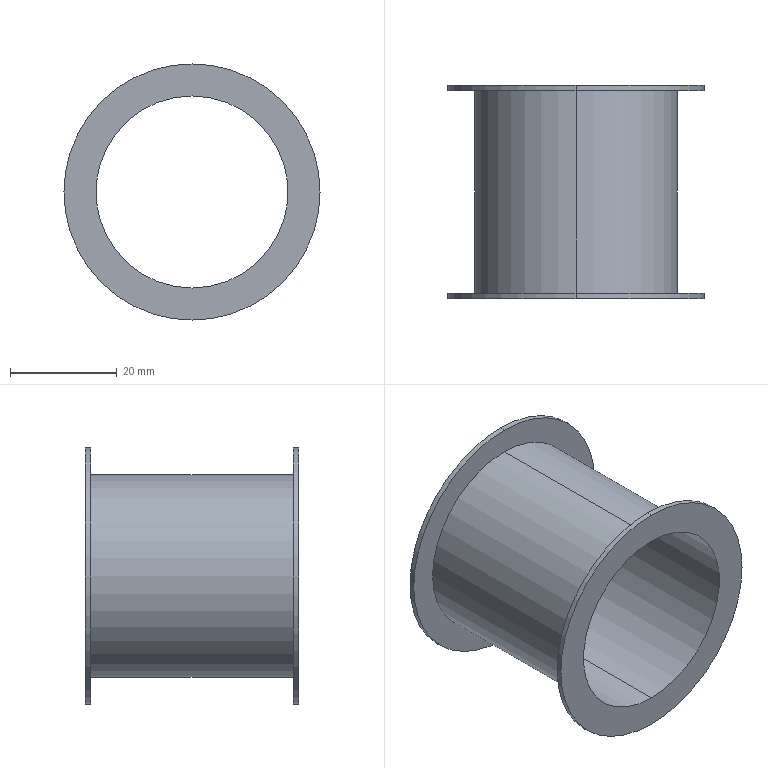Part | SolidWorks | features Revolution 1 | 1 solid | 12 faces | box 48 x 40 x 48 mm | volume 6000 mm3 | cylinder 8 | plane 4 | commonest cylinder face diameters 48 x4 36 x2 38 x2
STEP:
#1=CARTESIAN_POINT('',(0.,40.,-24.));
#2=VERTEX_POINT('',#1);
#3=CARTESIAN_POINT('',(0.,40.,24.));
#4=VERTEX_POINT('',#3);
#5=CARTESIAN_POINT('',(0.,40.,0.));
#6=DIRECTION('',(0.,-1.,0.));
#7=DIRECTION('',(0.,0.,-1.));
#8=AXIS2_PLACEMENT_3D('',#5,#6,#7);
#9=CIRCLE('',#8,24.);
#10=EDGE_CURVE('',#2,#4,#9,.T.);
#11=ORIENTED_EDGE('',*,*,#10,.T.);
#12=CARTESIAN_POINT('',(0.,39.,24.));
#13=VERTEX_POINT('',#12);
#14=CARTESIAN_POINT('',(0.,0.,24.));
#15=DIRECTION('',(0.,-1.,0.));
#16=VECTOR('',#15,1000.);
#17=LINE('',#14,#16);
#18=EDGE_CURVE('',#4,#13,#17,.T.);
#19=ORIENTED_EDGE('',*,*,#18,.T.);
#20=CARTESIAN_POINT('',(0.,39.,-24.));
#21=VERTEX_POINT('',#20);
#22=CARTESIAN_POINT('',(0.,39.,0.));
#23=DIRECTION('',(0.,-1.,0.));
#24=DIRECTION('',(0.,0.,-1.));
#25=AXIS2_PLACEMENT_3D('',#22,#23,#24);
#26=CIRCLE('',#25,24.);
#27=EDGE_CURVE('',#21,#13,#26,.T.);
#28=ORIENTED_EDGE('',*,*,#27,.F.);
#29=CARTESIAN_POINT('',(0.,0.,-24.));
#30=DIRECTION('',(0.,-1.,0.));
#31=VECTOR('',#30,1000.);
#32=LINE('',#29,#31);
#33=EDGE_CURVE('',#2,#21,#32,.T.);
#34=ORIENTED_EDGE('',*,*,#33,.F.);
#35=EDGE_LOOP('',(#11,#19,#28,#34));
#36=FACE_OUTER_BOUND('',#35,.T.);
#37=CARTESIAN_POINT('',(0.,0.,0.));
#38=DIRECTION('',(0.,-1.,0.));
#39=DIRECTION('',(0.,0.,-1.));
#40=AXIS2_PLACEMENT_3D('',#37,#38,#39);
#41=CYLINDRICAL_SURFACE('',#40,24.);
#42=ADVANCED_FACE('',(#36),#41,.T.);
#43=CARTESIAN_POINT('',(0.,39.,-19.));
#44=VERTEX_POINT('',#43);
#45=CARTESIAN_POINT('',(0.,39.,19.));
#46=VERTEX_POINT('',#45);
#47=CARTESIAN_POINT('',(0.,39.,0.));
#48=DIRECTION('',(0.,-1.,0.));
#49=DIRECTION('',(0.,0.,-1.));
#50=AXIS2_PLACEMENT_3D('',#47,#48,#49);
#51=CIRCLE('',#50,19.);
#52=EDGE_CURVE('',#44,#46,#51,.T.);
#53=ORIENTED_EDGE('',*,*,#52,.T.);
#54=CARTESIAN_POINT('',(0.,1.,19.));
#55=VERTEX_POINT('',#54);
#56=CARTESIAN_POINT('',(0.,0.,19.));
#57=DIRECTION('',(0.,-1.,0.));
#58=VECTOR('',#57,1000.);
#59=LINE('',#56,#58);
#60=EDGE_CURVE('',#46,#55,#59,.T.);
#61=ORIENTED_EDGE('',*,*,#60,.T.);
#62=CARTESIAN_POINT('',(0.,1.,-19.));
#63=VERTEX_POINT('',#62);
#64=CARTESIAN_POINT('',(0.,1.,0.));
#65=DIRECTION('',(0.,-1.,0.));
#66=DIRECTION('',(0.,0.,-1.));
#67=AXIS2_PLACEMENT_3D('',#64,#65,#66);
#68=CIRCLE('',#67,19.);
#69=EDGE_CURVE('',#63,#55,#68,.T.);
#70=ORIENTED_EDGE('',*,*,#69,.F.);
#71=CARTESIAN_POINT('',(0.,0.,-19.));
#72=DIRECTION('',(0.,-1.,0.));
#73=VECTOR('',#72,1000.);
#74=LINE('',#71,#73);
#75=EDGE_CURVE('',#44,#63,#74,.T.);
#76=ORIENTED_EDGE('',*,*,#75,.F.);
#77=EDGE_LOOP('',(#53,#61,#70,#76));
#78=FACE_OUTER_BOUND('',#77,.T.);
#79=CARTESIAN_POINT('',(0.,0.,0.));
#80=DIRECTION('',(0.,-1.,0.));
#81=DIRECTION('',(0.,0.,-1.));
#82=AXIS2_PLACEMENT_3D('',#79,#80,#81);
#83=CYLINDRICAL_SURFACE('',#82,19.);
#84=ADVANCED_FACE('',(#78),#83,.T.);
#85=CARTESIAN_POINT('',(0.,1.,-24.));
#86=VERTEX_POINT('',#85);
#87=CARTESIAN_POINT('',(0.,1.,24.));
#88=VERTEX_POINT('',#87);
#89=CARTESIAN_POINT('',(0.,1.,0.));
#90=DIRECTION('',(0.,-1.,0.));
#91=DIRECTION('',(0.,0.,-1.));
#92=AXIS2_PLACEMENT_3D('',#89,#90,#91);
#93=CIRCLE('',#92,24.);
#94=EDGE_CURVE('',#86,#88,#93,.T.);
#95=ORIENTED_EDGE('',*,*,#94,.T.);
#96=CARTESIAN_POINT('',(0.,0.,24.));
#97=VERTEX_POINT('',#96);
#98=CARTESIAN_POINT('',(0.,0.,24.));
#99=DIRECTION('',(0.,-1.,0.));
#100=VECTOR('',#99,1000.);
#101=LINE('',#98,#100);
#102=EDGE_CURVE('',#88,#97,#101,.T.);
#103=ORIENTED_EDGE('',*,*,#102,.T.);
#104=CARTESIAN_POINT('',(0.,0.,-24.));
#105=VERTEX_POINT('',#104);
#106=CARTESIAN_POINT('',(0.,0.,0.));
#107=DIRECTION('',(0.,-1.,0.));
#108=DIRECTION('',(0.,0.,-1.));
#109=AXIS2_PLACEMENT_3D('',#106,#107,#108);
#110=CIRCLE('',#109,24.);
#111=EDGE_CURVE('',#105,#97,#110,.T.);
#112=ORIENTED_EDGE('',*,*,#111,.F.);
#113=CARTESIAN_POINT('',(0.,0.,-24.));
#114=DIRECTION('',(0.,-1.,0.));
#115=VECTOR('',#114,1000.);
#116=LINE('',#113,#115);
#117=EDGE_CURVE('',#86,#105,#116,.T.);
#118=ORIENTED_EDGE('',*,*,#117,.F.);
#119=EDGE_LOOP('',(#95,#103,#112,#118));
#120=FACE_OUTER_BOUND('',#119,.T.);
#121=CARTESIAN_POINT('',(0.,0.,0.));
#122=DIRECTION('',(0.,-1.,0.));
#123=DIRECTION('',(0.,0.,-1.));
#124=AXIS2_PLACEMENT_3D('',#121,#122,#123);
#125=CYLINDRICAL_SURFACE('',#124,24.);
#126=ADVANCED_FACE('',(#120),#125,.T.);
#127=CARTESIAN_POINT('',(0.,40.,18.));
#128=VERTEX_POINT('',#127);
#129=CARTESIAN_POINT('',(0.,40.,-18.));
#130=VERTEX_POINT('',#129);
#131=CARTESIAN_POINT('',(0.,40.,0.));
#132=DIRECTION('',(0.,-1.,0.));
#133=DIRECTION('',(0.,0.,-1.));
#134=AXIS2_PLACEMENT_3D('',#131,#132,#133);
#135=CIRCLE('',#134,18.);
#136=EDGE_CURVE('',#128,#130,#135,.T.);
#137=ORIENTED_EDGE('',*,*,#136,.F.);
#138=CARTESIAN_POINT('',(0.,0.,18.));
#139=VERTEX_POINT('',#138);
#140=CARTESIAN_POINT('',(0.,0.,18.));
#141=DIRECTION('',(0.,-1.,0.));
#142=VECTOR('',#141,1000.);
#143=LINE('',#140,#142);
#144=EDGE_CURVE('',#128,#139,#143,.T.);
#145=ORIENTED_EDGE('',*,*,#144,.T.);
#146=CARTESIAN_POINT('',(0.,0.,-18.));
#147=VERTEX_POINT('',#146);
#148=CARTESIAN_POINT('',(0.,0.,0.));
#149=DIRECTION('',(0.,-1.,0.));
#150=DIRECTION('',(0.,0.,-1.));
#151=AXIS2_PLACEMENT_3D('',#148,#149,#150);
#152=CIRCLE('',#151,18.);
#153=EDGE_CURVE('',#139,#147,#152,.T.);
#154=ORIENTED_EDGE('',*,*,#153,.T.);
#155=CARTESIAN_POINT('',(0.,0.,-18.));
#156=DIRECTION('',(0.,-1.,0.));
#157=VECTOR('',#156,1000.);
#158=LINE('',#155,#157);
#159=EDGE_CURVE('',#130,#147,#158,.T.);
#160=ORIENTED_EDGE('',*,*,#159,.F.);
#161=EDGE_LOOP('',(#137,#145,#154,#160));
#162=FACE_OUTER_BOUND('',#161,.T.);
#163=CARTESIAN_POINT('',(0.,0.,0.));
#164=DIRECTION('',(0.,-1.,0.));
#165=DIRECTION('',(0.,0.,-1.));
#166=AXIS2_PLACEMENT_3D('',#163,#164,#165);
#167=CYLINDRICAL_SURFACE('',#166,18.);
#168=ADVANCED_FACE('',(#162),#167,.F.);
#169=CARTESIAN_POINT('',(0.,40.,0.));
#170=DIRECTION('',(0.,-1.,0.));
#171=DIRECTION('',(0.,0.,-1.));
#172=AXIS2_PLACEMENT_3D('',#169,#170,#171);
#173=CIRCLE('',#172,18.);
#174=EDGE_CURVE('',#130,#128,#173,.T.);
#175=ORIENTED_EDGE('',*,*,#174,.T.);
#176=ORIENTED_EDGE('',*,*,#136,.T.);
#177=EDGE_LOOP('',(#175,#176));
#178=FACE_BOUND('',#177,.T.);
#179=ORIENTED_EDGE('',*,*,#10,.F.);
#180=CARTESIAN_POINT('',(0.,40.,0.));
#181=DIRECTION('',(0.,-1.,0.));
#182=DIRECTION('',(0.,0.,-1.));
#183=AXIS2_PLACEMENT_3D('',#180,#181,#182);
#184=CIRCLE('',#183,24.);
#185=EDGE_CURVE('',#4,#2,#184,.T.);
#186=ORIENTED_EDGE('',*,*,#185,.F.);
#187=EDGE_LOOP('',(#179,#186));
#188=FACE_OUTER_BOUND('',#187,.T.);
#189=CARTESIAN_POINT('',(0.,40.,-24.));
#190=DIRECTION('',(0.,1.,0.));
#191=DIRECTION('',(0.,0.,1.));
#192=AXIS2_PLACEMENT_3D('',#189,#190,#191);
#193=PLANE('',#192);
#194=ADVANCED_FACE('',(#178,#188),#193,.T.);
#195=ORIENTED_EDGE('',*,*,#144,.F.);
#196=ORIENTED_EDGE('',*,*,#174,.F.);
#197=ORIENTED_EDGE('',*,*,#159,.T.);
#198=CARTESIAN_POINT('',(0.,0.,0.));
#199=DIRECTION('',(0.,-1.,0.));
#200=DIRECTION('',(0.,0.,-1.));
#201=AXIS2_PLACEMENT_3D('',#198,#199,#200);
#202=CIRCLE('',#201,18.);
#203=EDGE_CURVE('',#147,#139,#202,.T.);
#204=ORIENTED_EDGE('',*,*,#203,.T.);
#205=EDGE_LOOP('',(#195,#196,#197,#204));
#206=FACE_OUTER_BOUND('',#205,.T.);
#207=CARTESIAN_POINT('',(0.,0.,0.));
#208=DIRECTION('',(0.,-1.,0.));
#209=DIRECTION('',(0.,0.,-1.));
#210=AXIS2_PLACEMENT_3D('',#207,#208,#209);
#211=CYLINDRICAL_SURFACE('',#210,18.);
#212=ADVANCED_FACE('',(#206),#211,.F.);
#213=ORIENTED_EDGE('',*,*,#111,.T.);
#214=CARTESIAN_POINT('',(0.,0.,0.));
#215=DIRECTION('',(0.,-1.,0.));
#216=DIRECTION('',(0.,0.,-1.));
#217=AXIS2_PLACEMENT_3D('',#214,#215,#216);
#218=CIRCLE('',#217,24.);
#219=EDGE_CURVE('',#97,#105,#218,.T.);
#220=ORIENTED_EDGE('',*,*,#219,.T.);
#221=EDGE_LOOP('',(#213,#220));
#222=FACE_OUTER_BOUND('',#221,.T.);
#223=ORIENTED_EDGE('',*,*,#203,.F.);
#224=ORIENTED_EDGE('',*,*,#153,.F.);
#225=EDGE_LOOP('',(#223,#224));
#226=FACE_BOUND('',#225,.T.);
#227=CARTESIAN_POINT('',(0.,0.,-18.));
#228=DIRECTION('',(0.,-1.,0.));
#229=DIRECTION('',(0.,0.,-1.));
#230=AXIS2_PLACEMENT_3D('',#227,#228,#229);
#231=PLANE('',#230);
#232=ADVANCED_FACE('',(#222,#226),#231,.T.);
#233=ORIENTED_EDGE('',*,*,#102,.F.);
#234=CARTESIAN_POINT('',(0.,1.,0.));
#235=DIRECTION('',(0.,-1.,0.));
#236=DIRECTION('',(0.,0.,-1.));
#237=AXIS2_PLACEMENT_3D('',#234,#235,#236);
#238=CIRCLE('',#237,24.);
#239=EDGE_CURVE('',#88,#86,#238,.T.);
#240=ORIENTED_EDGE('',*,*,#239,.T.);
#241=ORIENTED_EDGE('',*,*,#117,.T.);
#242=ORIENTED_EDGE('',*,*,#219,.F.);
#243=EDGE_LOOP('',(#233,#240,#241,#242));
#244=FACE_OUTER_BOUND('',#243,.T.);
#245=CARTESIAN_POINT('',(0.,0.,0.));
#246=DIRECTION('',(0.,-1.,0.));
#247=DIRECTION('',(0.,0.,-1.));
#248=AXIS2_PLACEMENT_3D('',#245,#246,#247);
#249=CYLINDRICAL_SURFACE('',#248,24.);
#250=ADVANCED_FACE('',(#244),#249,.T.);
#251=ORIENTED_EDGE('',*,*,#94,.F.);
#252=ORIENTED_EDGE('',*,*,#239,.F.);
#253=EDGE_LOOP('',(#251,#252));
#254=FACE_OUTER_BOUND('',#253,.T.);
#255=ORIENTED_EDGE('',*,*,#69,.T.);
#256=CARTESIAN_POINT('',(0.,1.,0.));
#257=DIRECTION('',(0.,-1.,0.));
#258=DIRECTION('',(0.,0.,-1.));
#259=AXIS2_PLACEMENT_3D('',#256,#257,#258);
#260=CIRCLE('',#259,19.);
#261=EDGE_CURVE('',#55,#63,#260,.T.);
#262=ORIENTED_EDGE('',*,*,#261,.T.);
#263=EDGE_LOOP('',(#255,#262));
#264=FACE_BOUND('',#263,.T.);
#265=CARTESIAN_POINT('',(0.,1.,-19.));
#266=DIRECTION('',(0.,-1.,0.));
#267=DIRECTION('',(0.,0.,-1.));
#268=AXIS2_PLACEMENT_3D('',#265,#266,#267);
#269=PLANE('',#268);
#270=ADVANCED_FACE('',(#254,#264),#269,.F.);
#271=ORIENTED_EDGE('',*,*,#60,.F.);
#272=CARTESIAN_POINT('',(0.,39.,0.));
#273=DIRECTION('',(0.,-1.,0.));
#274=DIRECTION('',(0.,0.,-1.));
#275=AXIS2_PLACEMENT_3D('',#272,#273,#274);
#276=CIRCLE('',#275,19.);
#277=EDGE_CURVE('',#46,#44,#276,.T.);
#278=ORIENTED_EDGE('',*,*,#277,.T.);
#279=ORIENTED_EDGE('',*,*,#75,.T.);
#280=ORIENTED_EDGE('',*,*,#261,.F.);
#281=EDGE_LOOP('',(#271,#278,#279,#280));
#282=FACE_OUTER_BOUND('',#281,.T.);
#283=CARTESIAN_POINT('',(0.,0.,0.));
#284=DIRECTION('',(0.,-1.,0.));
#285=DIRECTION('',(0.,0.,-1.));
#286=AXIS2_PLACEMENT_3D('',#283,#284,#285);
#287=CYLINDRICAL_SURFACE('',#286,19.);
#288=ADVANCED_FACE('',(#282),#287,.T.);
#289=ORIENTED_EDGE('',*,*,#52,.F.);
#290=ORIENTED_EDGE('',*,*,#277,.F.);
#291=EDGE_LOOP('',(#289,#290));
#292=FACE_BOUND('',#291,.T.);
#293=ORIENTED_EDGE('',*,*,#27,.T.);
#294=CARTESIAN_POINT('',(0.,39.,0.));
#295=DIRECTION('',(0.,-1.,0.));
#296=DIRECTION('',(0.,0.,-1.));
#297=AXIS2_PLACEMENT_3D('',#294,#295,#296);
#298=CIRCLE('',#297,24.);
#299=EDGE_CURVE('',#13,#21,#298,.T.);
#300=ORIENTED_EDGE('',*,*,#299,.T.);
#301=EDGE_LOOP('',(#293,#300));
#302=FACE_OUTER_BOUND('',#301,.T.);
#303=CARTESIAN_POINT('',(0.,39.,-24.));
#304=DIRECTION('',(0.,1.,0.));
#305=DIRECTION('',(0.,0.,1.));
#306=AXIS2_PLACEMENT_3D('',#303,#304,#305);
#307=PLANE('',#306);
#308=ADVANCED_FACE('',(#292,#302),#307,.F.);
#309=ORIENTED_EDGE('',*,*,#18,.F.);
#310=ORIENTED_EDGE('',*,*,#185,.T.);
#311=ORIENTED_EDGE('',*,*,#33,.T.);
#312=ORIENTED_EDGE('',*,*,#299,.F.);
#313=EDGE_LOOP('',(#309,#310,#311,#312));
#314=FACE_OUTER_BOUND('',#313,.T.);
#315=CARTESIAN_POINT('',(0.,0.,0.));
#316=DIRECTION('',(0.,-1.,0.));
#317=DIRECTION('',(0.,0.,-1.));
#318=AXIS2_PLACEMENT_3D('',#315,#316,#317);
#319=CYLINDRICAL_SURFACE('',#318,24.);
#320=ADVANCED_FACE('',(#314),#319,.T.);
#321=CLOSED_SHELL('',(#42,#84,#126,#168,#194,#212,#232,#250,#270,#288,#308,#320));
#322=MANIFOLD_SOLID_BREP('',#321);
#323=CARTESIAN_POINT('',(0.,0.,0.));
#324=DIRECTION('',(0.,0.,1.));
#325=DIRECTION('',(1.,0.,0.));
#326=AXIS2_PLACEMENT_3D('',#323,#324,#325);
#327=(LENGTH_UNIT()NAMED_UNIT(*)SI_UNIT(.MILLI.,.METRE.));
#328=UNCERTAINTY_MEASURE_WITH_UNIT(LENGTH_MEASURE(0.00001),#327,'','');
#329=(NAMED_UNIT(*)PLANE_ANGLE_UNIT()SI_UNIT($,.RADIAN.));
#330=(NAMED_UNIT(*)SI_UNIT($,.STERADIAN.)SOLID_ANGLE_UNIT());
#331=(GEOMETRIC_REPRESENTATION_CONTEXT(3)GLOBAL_UNCERTAINTY_ASSIGNED_CONTEXT((#328))GLOBAL_UNIT_ASSIGNED_CONTEXT((#327,#329,#330))REPRESENTATION_CONTEXT('',''));
#332=ADVANCED_BREP_SHAPE_REPRESENTATION('',(#322,#326),#331);